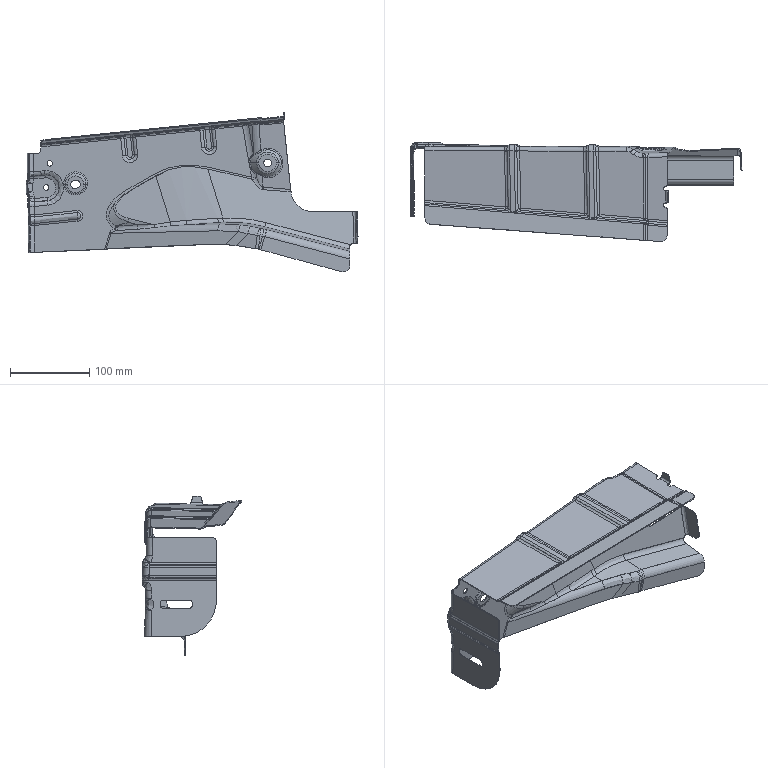Part | 1 solid | 561 faces | box 417.748 x 125.062 x 201.294 mm | volume 123548 mm3 | spline 308 | cylinder 157 | plane 71 | sphere 20 | other 3 | torus 2 | commonest cylinder face diameters 10 x42 7.6 x23 12.4 x17 16 x11 6 x8 13.6 x8